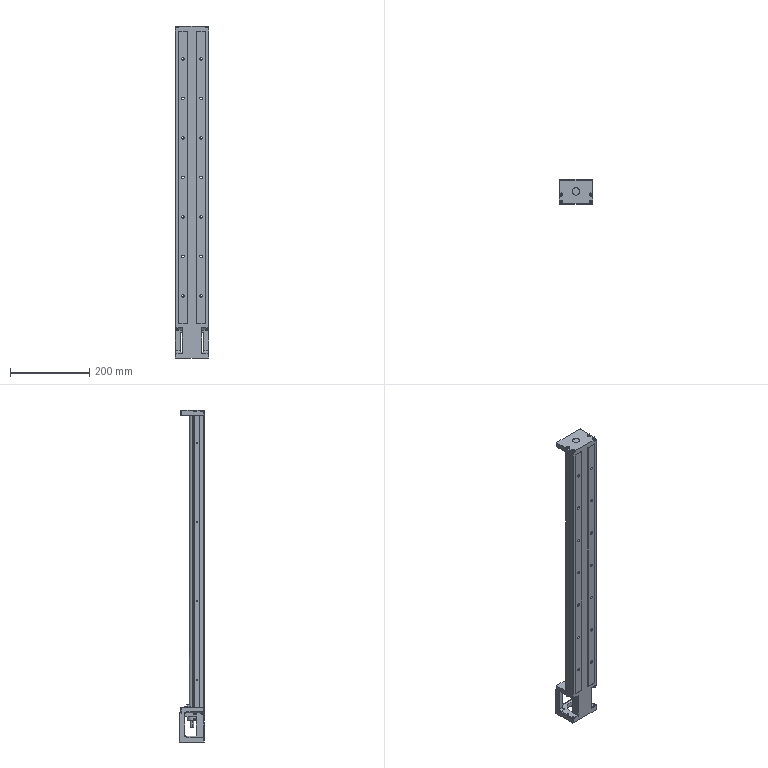Part | SolidWorks | features BaseBody 1 | 1 solid | 465 faces | box 86 x 64 x 840 mm | volume 1374741 mm3 | plane 226 | cylinder 207 | cone 18 | spline 14 | commonest cylinder face diameters 3 x31 6.6 x28 11 x28 7.5 x24 2.15 x16 3.3 x16